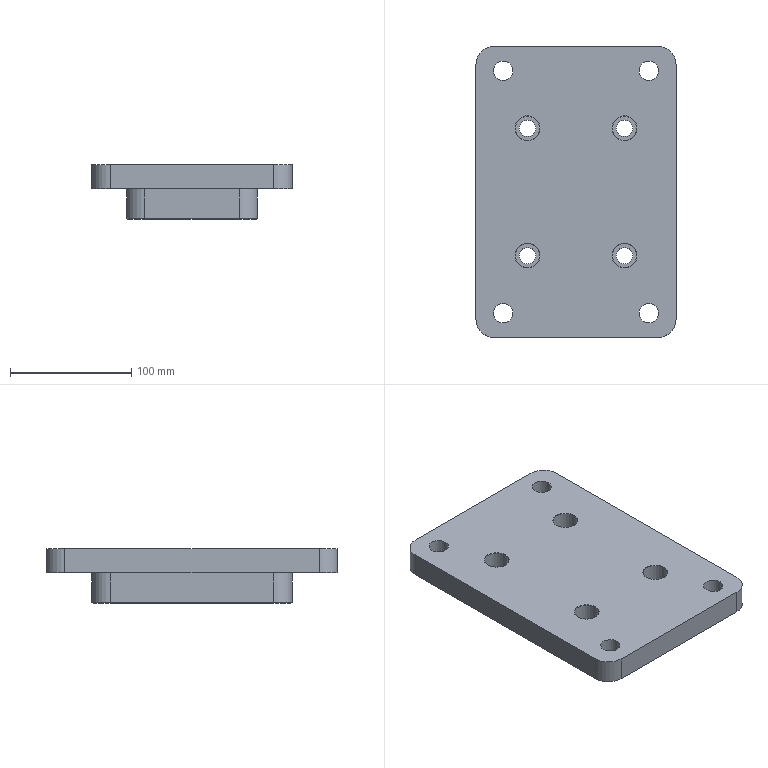NC program | NX | posted with a generic post | part box 165 x 240 x 45 mm
Lines 5642 to 5916 of 5916:
(HOLE_MILLING_COPY , TOOL : D10JING)
N11264 T11 M6
N11266 G54
N11268 G17 G0 G90 X-100. Y60. S5000 M3
N11270 G43 Z30. H11
N11272 Z0.5
N11274 G94 G3 X-101.5 Y58.5 R1.5 F1200.
N11276 X-100. Y57. R1.5
N11278 X-100. Y57. Z-4.5 I0. J3.
N11280 X-100. Y57. Z-9.5 I0. J3.
N11282 X-100. Y57. Z-14.5 I0. J3.
N11284 X-100. Y57. Z-19.5 I0. J3.
N11286 X-98.237 Y57.573 Z-20. R3.
N11288 X-97.573 Y61.763 R3.
N11290 X-98.237 Y57.573 R-3.
N11292 X-97.905 Y59.668 R1.5
N11294 X-100. Y60. R1.5
N11296 G0 Z30.
N11298 X-52.5 Y40.
N11300 Z0.5
N11302 G1 X-53.935 Y38.68
N11304 G3 X-52.5 Y35. R2.12
N11306 X-52.5 Y35. Z-4.5 I0. J5.
N11308 X-52.5 Y35. Z-9.5 I0. J5.
N11310 X-52.5 Y35. Z-14.5 I0. J5.
N11312 X-57.255 Y41.545 Z-18. R-5.
N11314 X-54.045 Y35.245 R5.
N11316 X-57.255 Y41.545 R-5.
N11318 X-54.199 Y39.043 R2.12
N11320 G1 X-52.5 Y40.
N11322 G0 Z30.
N11324 X-100. Y-60.
N11326 Z0.5
N11328 G3 X-101.5 Y-61.5 R1.5
N11330 X-100. Y-63. R1.5
N11332 X-100. Y-63. Z-4.5 I0. J3.
N11334 X-100. Y-63. Z-9.5 I0. J3.
N11336 X-100. Y-63. Z-14.5 I0. J3.
N11338 X-100. Y-63. Z-19.5 I0. J3.
N11340 X-98.237 Y-62.427 Z-20. R3.
N11342 X-97.573 Y-58.237 R3.
N11344 X-98.237 Y-62.427 R-3.
N11346 X-97.905 Y-60.332 R1.5
N11348 X-100. Y-60. R1.5
N11350 G0 Z30.
N11352 X-52.5 Y-40.
N11354 Z0.5
N11356 G1 X-53.935 Y-41.32
N11358 G3 X-52.5 Y-45. R2.12
N11360 X-52.5 Y-45. Z-4.5 I0. J5.
N11362 X-52.5 Y-45. Z-9.5 I0. J5.
N11364 X-52.5 Y-45. Z-14.5 I0. J5.
N11366 X-57.255 Y-38.455 Z-18. R-5.
N11368 X-54.045 Y-44.755 R5.
N11370 X-57.255 Y-38.455 R-5.
N11372 X-54.199 Y-40.957 R2.12
N11374 G1 X-52.5 Y-40.
N11376 G0 Z30.
N11378 X52.5
N11380 Z0.5
N11382 G1 X51.065 Y-41.32
N11384 G3 X52.5 Y-45. R2.12
N11386 X52.5 Y-45. Z-4.5 I0. J5.
N11388 X52.5 Y-45. Z-9.5 I0. J5.
N11390 X52.5 Y-45. Z-14.5 I0. J5.
N11392 X47.745 Y-38.455 Z-18. R-5.
N11394 X50.955 Y-44.755 R5.
N11396 X47.745 Y-38.455 R-5.
N11398 X50.801 Y-40.957 R2.12
N11400 G1 X52.5 Y-40.
N11402 G0 Z30.
N11404 X100. Y-60.
N11406 Z0.5
N11408 G3 X98.5 Y-61.5 R1.5
N11410 X100. Y-63. R1.5
N11412 X100. Y-63. Z-4.5 I0. J3.
N11414 X100. Y-63. Z-9.5 I0. J3.
N11416 X100. Y-63. Z-14.5 I0. J3.
N11418 X100. Y-63. Z-19.5 I0. J3.
N11420 X101.763 Y-62.427 Z-20. R3.
N11422 X102.427 Y-58.237 R3.
N11424 X101.763 Y-62.427 R-3.
N11426 X102.095 Y-60.332 R1.5
N11428 X100. Y-60. R1.5
N11430 G0 Z30.
N11432 X52.5 Y40.
N11434 Z0.5
N11436 G1 X51.065 Y38.68
N11438 G3 X52.5 Y35. R2.12
N11440 X52.5 Y35. Z-4.5 I0. J5.
N11442 X52.5 Y35. Z-9.5 I0. J5.
N11444 X52.5 Y35. Z-14.5 I0. J5.
N11446 X47.745 Y41.545 Z-18. R-5.
N11448 X50.955 Y35.245 R5.
N11450 X47.745 Y41.545 R-5.
N11452 X50.801 Y39.043 R2.12
N11454 G1 X52.5 Y40.
N11456 G0 Z30.
N11458 X100. Y60.
N11460 Z0.5
N11462 G3 X98.5 Y58.5 R1.5
N11464 X100. Y57. R1.5
N11466 X100. Y57. Z-4.5 I0. J3.
N11468 X100. Y57. Z-9.5 I0. J3.
N11470 X100. Y57. Z-14.5 I0. J3.
N11472 X100. Y57. Z-19.5 I0. J3.
N11474 X101.763 Y57.573 Z-20. R3.
N11476 X102.427 Y61.763 R3.
N11478 X101.763 Y57.573 R-3.
N11480 X102.095 Y59.668 R1.5
N11482 X100. Y60. R1.5
N11484 G0 Z30.
(ZLEVEL_PROFILE_1 , TOOL : D10JING)
N11486 X127. Y-60.375
N11488 Z-16.
N11490 G1 Z-18. F1250.
N11492 X125.499 Y-61.242
N11494 G3 X124.999 Y-62.108 R1.
N11496 G1 X125. Y-66.998
N11498 Y-67.5
N11500 G2 X105. Y-87.5 R20.
N11502 G1 X104.498
N11504 X99.608 Y-87.499
N11506 G3 X98.742 Y-87.999 R1.
N11508 G1 X97.875 Y-89.5
N11510 Z-16.
N11512 G0 Z30.
N11514 Y89.5
N11516 Z-16.
N11518 G1 Z-18.
N11520 X98.742 Y87.999
N11522 G3 X99.608 Y87.499 R1.
N11524 G1 X104.053
N11526 X104.498 Y87.5
N11528 X105.
N11530 G2 X125. Y67.5 R20.
N11532 G1 Y66.998
N11534 X124.999 Y62.108
N11536 G3 X125.499 Y61.242 R1.
N11538 G1 X127. Y60.375
N11540 Z-16.
N11542 G0 Z30.
N11544 X-127.
N11546 Z-16.
N11548 G1 Z-18.
N11550 X-125.499 Y61.242
N11552 G3 X-124.999 Y62.108 R1.
N11554 G1 Y66.553
N11556 X-125. Y66.998
N11558 Y67.5
N11560 G2 X-105. Y87.5 R20.
N11562 G1 X-104.498
N11564 X-104.053 Y87.499
N11566 X-99.608
N11568 G3 X-98.742 Y87.999 R1.
N11570 G1 X-97.875 Y89.5
N11572 Z-16.
N11574 G0 Z30.
N11576 Y-89.5
N11578 Z-16.
N11580 G1 Z-18.
N11582 X-98.742 Y-87.999
N11584 G3 X-99.608 Y-87.499 R1.
N11586 G1 X-104.498 Y-87.5
N11588 X-105.
N11590 G2 X-125. Y-67.512 R20.
N11592 G1 Y-67.481
N11594 Y-66.998
N11596 X-124.999 Y-66.553
N11598 Y-62.108
N11600 G3 X-125.499 Y-61.242 R1.
N11602 G1 X-127. Y-60.375
N11604 Z-16.
N11606 G0 Z30.
N11608 M5
(PLANAR_MILL_COPY_COPY , TOOL : D6A45)
N11610 T07 M6
N11612 G54
N11614 G17 G0 G90 X100.766 Y66.343 S7500 M3
N11616 G43 Z30. H7
N11618 Z1.5
N11620 G94 G1 Z-1.5 F1250.
N11622 G3 X100. Y66.7 R1.
N11624 X93.3 Y60. R6.7
N11626 X100. Y66.7 R-6.7
N11628 X99.234 Y66.343 R1.
N11630 G1 Z1.5
N11632 G0 Z30.
N11634 X53.266 Y48.593
N11636 Z1.5
N11638 G1 Z-1.5
N11640 G3 X52.5 Y48.95 R1.
N11642 X43.55 Y40. R8.95
N11644 X52.5 Y48.95 R-8.95
N11646 X51.734 Y48.593 R1.
N11648 G1 Z1.5
N11650 G0 Z30.
N11652 X106.343 Y-60.766
N11654 Z1.5
N11656 G1 Z-1.5
N11658 G3 X106.7 Y-60. R1.
N11660 X100. Y-53.3 R6.7
N11662 X106.7 Y-60. R-6.7
N11664 X106.343 Y-59.234 R1.
N11666 G1 Z1.5
N11668 G0 Z30.
N11670 X51.734 Y-48.593
N11672 Z1.5
N11674 G1 Z-1.5
N11676 G3 X52.5 Y-48.95 R1.
N11678 X61.45 Y-40. R8.95
N11680 X52.5 Y-48.95 R-8.95
N11682 X53.266 Y-48.593 R1.
N11684 G1 Z1.5
N11686 G0 Z30.
N11688 X0.766 Y-84.157
N11690 Z1.5
N11692 G1 Z-1.5
N11694 G3 X0. Y-83.8 R1.
N11696 G1 X-105.
N11698 G2 X-121.3 Y-67.5 R16.3
N11700 G1 Y67.5
N11702 G2 X-105. Y83.8 R16.3
N11704 G1 X105.
N11706 G2 X121.3 Y67.5 R16.3
N11708 G1 Y-67.5
N11710 G2 X105. Y-83.8 R16.3
N11712 G1 X0.
N11714 G3 X-0.766 Y-84.157 R1.
N11716 G1 Z1.5
N11718 G0 Z30.
N11720 X-53.266 Y-48.593
N11722 Z1.5
N11724 G1 Z-1.5
N11726 G3 X-52.5 Y-48.95 R1.
N11728 X-43.55 Y-40. R8.95
N11730 X-52.5 Y-48.95 R-8.95
N11732 X-51.734 Y-48.593 R1.
N11734 G1 Z1.5
N11736 G0 Z30.
N11738 X-106.343 Y-59.234
N11740 Z1.5
N11742 G1 Z-1.5
N11744 G3 X-106.7 Y-60. R1.
N11746 X-100. Y-66.7 R6.7
N11748 X-106.7 Y-60. R-6.7
N11750 X-106.343 Y-60.766 R1.
N11752 G1 Z1.5
N11754 G0 Z30.
N11756 X-51.734 Y48.593
N11758 Z1.5
N11760 G1 Z-1.5
N11762 G3 X-52.5 Y48.95 R1.
N11764 X-61.45 Y40. R8.95
N11766 X-52.5 Y48.95 R-8.95
N11768 X-53.266 Y48.593 R1.
N11770 G1 Z1.5
N11772 G0 Z30.
N11774 X-106.343 Y60.766
N11776 Z1.5
N11778 G1 Z-1.5
N11780 G3 X-106.7 Y60. R1.
N11782 X-100. Y53.3 R6.7
N11784 X-106.7 Y60. R-6.7
N11786 X-106.343 Y59.234 R1.
N11788 G1 Z1.5
N11790 G0 Z30.
N11792 M5
N11794 M2